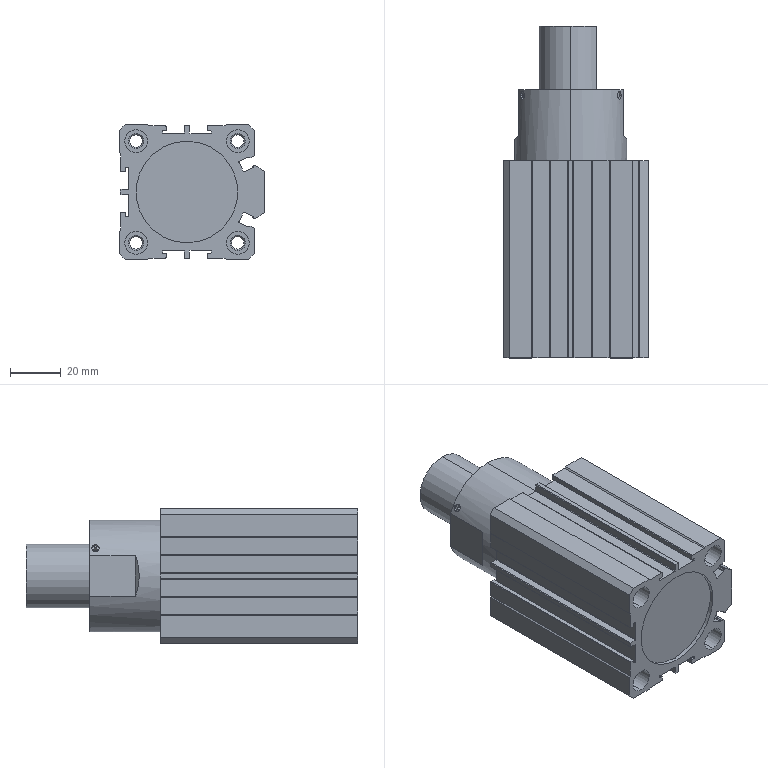Part | SolidWorks | 2 solids | 243 faces | box 57 x 130.5 x 53 mm | volume 211262 mm3 | plane 110 | cylinder 107 | cone 26 | commonest cylinder face diameters 0.4 x41 9 x16 0.8 x10 4.917 x8 3 x6 1 x5